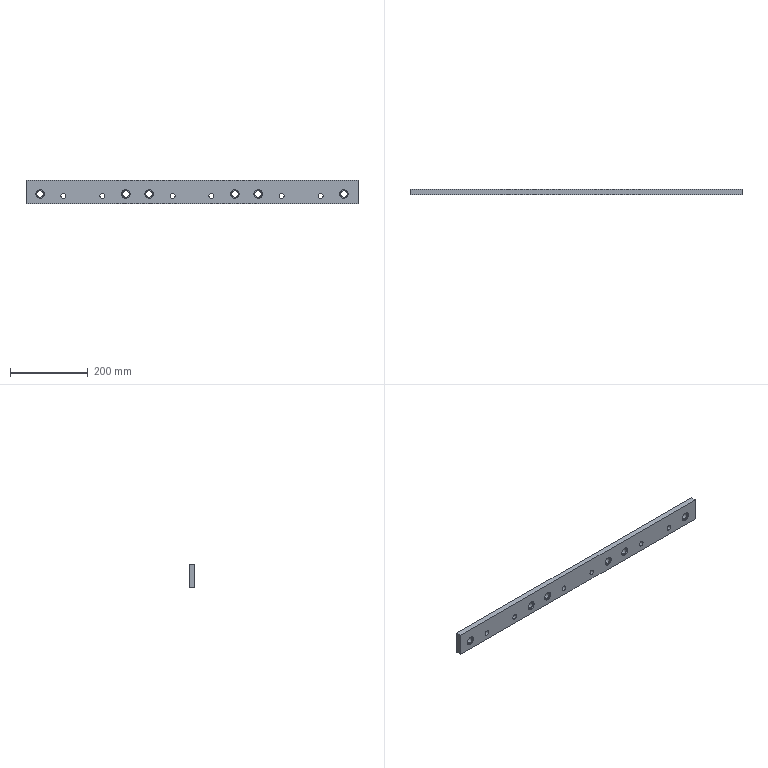Part | SolidWorks | features BaseBody 1 | 1 solid | 48 faces | box 852 x 14 x 60 mm | volume 682707 mm3 | cylinder 36 | plane 12 | commonest cylinder face diameters 13 x12 17 x12 22 x12
STEP:
#1=CARTESIAN_POINT('',(816.,3.,-43.5));
#2=VERTEX_POINT('',#1);
#3=CARTESIAN_POINT('',(816.,3.,-26.5));
#4=VERTEX_POINT('',#3);
#5=CARTESIAN_POINT('',(816.,3.,-35.));
#6=DIRECTION('',(0.,1.,0.));
#7=DIRECTION('',(0.,0.,1.));
#8=AXIS2_PLACEMENT_3D('',#5,#6,#7);
#9=CIRCLE('',#8,8.5);
#10=EDGE_CURVE('',#2,#4,#9,.T.);
#11=ORIENTED_EDGE('',*,*,#10,.F.);
#12=CARTESIAN_POINT('',(816.,14.,-43.5));
#13=VERTEX_POINT('',#12);
#14=CARTESIAN_POINT('',(816.,14.,-43.5));
#15=DIRECTION('',(0.,1.,0.));
#16=VECTOR('',#15,1000.);
#17=LINE('',#14,#16);
#18=EDGE_CURVE('',#2,#13,#17,.T.);
#19=ORIENTED_EDGE('',*,*,#18,.T.);
#20=CARTESIAN_POINT('',(816.,14.,-26.5));
#21=VERTEX_POINT('',#20);
#22=CARTESIAN_POINT('',(816.,14.,-35.));
#23=DIRECTION('',(0.,-1.,0.));
#24=DIRECTION('',(0.,0.,1.));
#25=AXIS2_PLACEMENT_3D('',#22,#23,#24);
#26=CIRCLE('',#25,8.5);
#27=EDGE_CURVE('',#21,#13,#26,.T.);
#28=ORIENTED_EDGE('',*,*,#27,.F.);
#29=CARTESIAN_POINT('',(816.,14.,-26.5));
#30=DIRECTION('',(0.,1.,0.));
#31=VECTOR('',#30,1000.);
#32=LINE('',#29,#31);
#33=EDGE_CURVE('',#4,#21,#32,.T.);
#34=ORIENTED_EDGE('',*,*,#33,.F.);
#35=EDGE_LOOP('',(#11,#19,#28,#34));
#36=FACE_OUTER_BOUND('',#35,.T.);
#37=CARTESIAN_POINT('',(816.,14.,-35.));
#38=DIRECTION('',(0.,1.,0.));
#39=DIRECTION('',(0.,0.,1.));
#40=AXIS2_PLACEMENT_3D('',#37,#38,#39);
#41=CYLINDRICAL_SURFACE('',#40,8.5);
#42=ADVANCED_FACE('',(#36),#41,.F.);
#43=CARTESIAN_POINT('',(536.,3.,-43.5));
#44=VERTEX_POINT('',#43);
#45=CARTESIAN_POINT('',(536.,3.,-26.5));
#46=VERTEX_POINT('',#45);
#47=CARTESIAN_POINT('',(536.,3.,-35.));
#48=DIRECTION('',(0.,1.,0.));
#49=DIRECTION('',(0.,0.,1.));
#50=AXIS2_PLACEMENT_3D('',#47,#48,#49);
#51=CIRCLE('',#50,8.5);
#52=EDGE_CURVE('',#44,#46,#51,.T.);
#53=ORIENTED_EDGE('',*,*,#52,.F.);
#54=CARTESIAN_POINT('',(536.,14.,-43.5));
#55=VERTEX_POINT('',#54);
#56=CARTESIAN_POINT('',(536.,14.,-43.5));
#57=DIRECTION('',(0.,1.,0.));
#58=VECTOR('',#57,1000.);
#59=LINE('',#56,#58);
#60=EDGE_CURVE('',#44,#55,#59,.T.);
#61=ORIENTED_EDGE('',*,*,#60,.T.);
#62=CARTESIAN_POINT('',(536.,14.,-26.5));
#63=VERTEX_POINT('',#62);
#64=CARTESIAN_POINT('',(536.,14.,-35.));
#65=DIRECTION('',(0.,-1.,0.));
#66=DIRECTION('',(0.,0.,1.));
#67=AXIS2_PLACEMENT_3D('',#64,#65,#66);
#68=CIRCLE('',#67,8.5);
#69=EDGE_CURVE('',#63,#55,#68,.T.);
#70=ORIENTED_EDGE('',*,*,#69,.F.);
#71=CARTESIAN_POINT('',(536.,14.,-26.5));
#72=DIRECTION('',(0.,1.,0.));
#73=VECTOR('',#72,1000.);
#74=LINE('',#71,#73);
#75=EDGE_CURVE('',#46,#63,#74,.T.);
#76=ORIENTED_EDGE('',*,*,#75,.F.);
#77=EDGE_LOOP('',(#53,#61,#70,#76));
#78=FACE_OUTER_BOUND('',#77,.T.);
#79=CARTESIAN_POINT('',(536.,14.,-35.));
#80=DIRECTION('',(0.,1.,0.));
#81=DIRECTION('',(0.,0.,1.));
#82=AXIS2_PLACEMENT_3D('',#79,#80,#81);
#83=CYLINDRICAL_SURFACE('',#82,8.5);
#84=ADVANCED_FACE('',(#78),#83,.F.);
#85=CARTESIAN_POINT('',(256.,3.,-43.5));
#86=VERTEX_POINT('',#85);
#87=CARTESIAN_POINT('',(256.,3.,-26.5));
#88=VERTEX_POINT('',#87);
#89=CARTESIAN_POINT('',(256.,3.,-35.));
#90=DIRECTION('',(0.,1.,0.));
#91=DIRECTION('',(0.,0.,1.));
#92=AXIS2_PLACEMENT_3D('',#89,#90,#91);
#93=CIRCLE('',#92,8.5);
#94=EDGE_CURVE('',#86,#88,#93,.T.);
#95=ORIENTED_EDGE('',*,*,#94,.F.);
#96=CARTESIAN_POINT('',(256.,14.,-43.5));
#97=VERTEX_POINT('',#96);
#98=CARTESIAN_POINT('',(256.,14.,-43.5));
#99=DIRECTION('',(0.,1.,0.));
#100=VECTOR('',#99,1000.);
#101=LINE('',#98,#100);
#102=EDGE_CURVE('',#86,#97,#101,.T.);
#103=ORIENTED_EDGE('',*,*,#102,.T.);
#104=CARTESIAN_POINT('',(256.,14.,-26.5));
#105=VERTEX_POINT('',#104);
#106=CARTESIAN_POINT('',(256.,14.,-35.));
#107=DIRECTION('',(0.,-1.,0.));
#108=DIRECTION('',(0.,0.,1.));
#109=AXIS2_PLACEMENT_3D('',#106,#107,#108);
#110=CIRCLE('',#109,8.5);
#111=EDGE_CURVE('',#105,#97,#110,.T.);
#112=ORIENTED_EDGE('',*,*,#111,.F.);
#113=CARTESIAN_POINT('',(256.,14.,-26.5));
#114=DIRECTION('',(0.,1.,0.));
#115=VECTOR('',#114,1000.);
#116=LINE('',#113,#115);
#117=EDGE_CURVE('',#88,#105,#116,.T.);
#118=ORIENTED_EDGE('',*,*,#117,.F.);
#119=EDGE_LOOP('',(#95,#103,#112,#118));
#120=FACE_OUTER_BOUND('',#119,.T.);
#121=CARTESIAN_POINT('',(256.,14.,-35.));
#122=DIRECTION('',(0.,1.,0.));
#123=DIRECTION('',(0.,0.,1.));
#124=AXIS2_PLACEMENT_3D('',#121,#122,#123);
#125=CYLINDRICAL_SURFACE('',#124,8.5);
#126=ADVANCED_FACE('',(#120),#125,.F.);
#127=CARTESIAN_POINT('',(756.,0.,-46.5));
#128=VERTEX_POINT('',#127);
#129=CARTESIAN_POINT('',(756.,0.,-33.5));
#130=VERTEX_POINT('',#129);
#131=CARTESIAN_POINT('',(756.,0.,-40.));
#132=DIRECTION('',(0.,1.,0.));
#133=DIRECTION('',(0.,0.,1.));
#134=AXIS2_PLACEMENT_3D('',#131,#132,#133);
#135=CIRCLE('',#134,6.5);
#136=EDGE_CURVE('',#128,#130,#135,.T.);
#137=ORIENTED_EDGE('',*,*,#136,.F.);
#138=CARTESIAN_POINT('',(756.,14.,-46.5));
#139=VERTEX_POINT('',#138);
#140=CARTESIAN_POINT('',(756.,14.,-46.5));
#141=DIRECTION('',(0.,1.,0.));
#142=VECTOR('',#141,1000.);
#143=LINE('',#140,#142);
#144=EDGE_CURVE('',#128,#139,#143,.T.);
#145=ORIENTED_EDGE('',*,*,#144,.T.);
#146=CARTESIAN_POINT('',(756.,14.,-33.5));
#147=VERTEX_POINT('',#146);
#148=CARTESIAN_POINT('',(756.,14.,-40.));
#149=DIRECTION('',(0.,-1.,0.));
#150=DIRECTION('',(0.,0.,1.));
#151=AXIS2_PLACEMENT_3D('',#148,#149,#150);
#152=CIRCLE('',#151,6.5);
#153=EDGE_CURVE('',#147,#139,#152,.T.);
#154=ORIENTED_EDGE('',*,*,#153,.F.);
#155=CARTESIAN_POINT('',(756.,14.,-33.5));
#156=DIRECTION('',(0.,1.,0.));
#157=VECTOR('',#156,1000.);
#158=LINE('',#155,#157);
#159=EDGE_CURVE('',#130,#147,#158,.T.);
#160=ORIENTED_EDGE('',*,*,#159,.F.);
#161=EDGE_LOOP('',(#137,#145,#154,#160));
#162=FACE_OUTER_BOUND('',#161,.T.);
#163=CARTESIAN_POINT('',(756.,14.,-40.));
#164=DIRECTION('',(0.,1.,0.));
#165=DIRECTION('',(0.,0.,1.));
#166=AXIS2_PLACEMENT_3D('',#163,#164,#165);
#167=CYLINDRICAL_SURFACE('',#166,6.5);
#168=ADVANCED_FACE('',(#162),#167,.F.);
#169=CARTESIAN_POINT('',(476.,0.,-46.5));
#170=VERTEX_POINT('',#169);
#171=CARTESIAN_POINT('',(476.,0.,-33.5));
#172=VERTEX_POINT('',#171);
#173=CARTESIAN_POINT('',(476.,0.,-40.));
#174=DIRECTION('',(0.,1.,0.));
#175=DIRECTION('',(0.,0.,1.));
#176=AXIS2_PLACEMENT_3D('',#173,#174,#175);
#177=CIRCLE('',#176,6.5);
#178=EDGE_CURVE('',#170,#172,#177,.T.);
#179=ORIENTED_EDGE('',*,*,#178,.F.);
#180=CARTESIAN_POINT('',(476.,14.,-46.5));
#181=VERTEX_POINT('',#180);
#182=CARTESIAN_POINT('',(476.,14.,-46.5));
#183=DIRECTION('',(0.,1.,0.));
#184=VECTOR('',#183,1000.);
#185=LINE('',#182,#184);
#186=EDGE_CURVE('',#170,#181,#185,.T.);
#187=ORIENTED_EDGE('',*,*,#186,.T.);
#188=CARTESIAN_POINT('',(476.,14.,-33.5));
#189=VERTEX_POINT('',#188);
#190=CARTESIAN_POINT('',(476.,14.,-40.));
#191=DIRECTION('',(0.,-1.,0.));
#192=DIRECTION('',(0.,0.,1.));
#193=AXIS2_PLACEMENT_3D('',#190,#191,#192);
#194=CIRCLE('',#193,6.5);
#195=EDGE_CURVE('',#189,#181,#194,.T.);
#196=ORIENTED_EDGE('',*,*,#195,.F.);
#197=CARTESIAN_POINT('',(476.,14.,-33.5));
#198=DIRECTION('',(0.,1.,0.));
#199=VECTOR('',#198,1000.);
#200=LINE('',#197,#199);
#201=EDGE_CURVE('',#172,#189,#200,.T.);
#202=ORIENTED_EDGE('',*,*,#201,.F.);
#203=EDGE_LOOP('',(#179,#187,#196,#202));
#204=FACE_OUTER_BOUND('',#203,.T.);
#205=CARTESIAN_POINT('',(476.,14.,-40.));
#206=DIRECTION('',(0.,1.,0.));
#207=DIRECTION('',(0.,0.,1.));
#208=AXIS2_PLACEMENT_3D('',#205,#206,#207);
#209=CYLINDRICAL_SURFACE('',#208,6.5);
#210=ADVANCED_FACE('',(#204),#209,.F.);
#211=CARTESIAN_POINT('',(196.,0.,-46.5));
#212=VERTEX_POINT('',#211);
#213=CARTESIAN_POINT('',(196.,0.,-33.5));
#214=VERTEX_POINT('',#213);
#215=CARTESIAN_POINT('',(196.,0.,-40.));
#216=DIRECTION('',(0.,1.,0.));
#217=DIRECTION('',(0.,0.,1.));
#218=AXIS2_PLACEMENT_3D('',#215,#216,#217);
#219=CIRCLE('',#218,6.5);
#220=EDGE_CURVE('',#212,#214,#219,.T.);
#221=ORIENTED_EDGE('',*,*,#220,.F.);
#222=CARTESIAN_POINT('',(196.,14.,-46.5));
#223=VERTEX_POINT('',#222);
#224=CARTESIAN_POINT('',(196.,14.,-46.5));
#225=DIRECTION('',(0.,1.,0.));
#226=VECTOR('',#225,1000.);
#227=LINE('',#224,#226);
#228=EDGE_CURVE('',#212,#223,#227,.T.);
#229=ORIENTED_EDGE('',*,*,#228,.T.);
#230=CARTESIAN_POINT('',(196.,14.,-33.5));
#231=VERTEX_POINT('',#230);
#232=CARTESIAN_POINT('',(196.,14.,-40.));
#233=DIRECTION('',(0.,-1.,0.));
#234=DIRECTION('',(0.,0.,1.));
#235=AXIS2_PLACEMENT_3D('',#232,#233,#234);
#236=CIRCLE('',#235,6.5);
#237=EDGE_CURVE('',#231,#223,#236,.T.);
#238=ORIENTED_EDGE('',*,*,#237,.F.);
#239=CARTESIAN_POINT('',(196.,14.,-33.5));
#240=DIRECTION('',(0.,1.,0.));
#241=VECTOR('',#240,1000.);
#242=LINE('',#239,#241);
#243=EDGE_CURVE('',#214,#231,#242,.T.);
#244=ORIENTED_EDGE('',*,*,#243,.F.);
#245=EDGE_LOOP('',(#221,#229,#238,#244));
#246=FACE_OUTER_BOUND('',#245,.T.);
#247=CARTESIAN_POINT('',(196.,14.,-40.));
#248=DIRECTION('',(0.,1.,0.));
#249=DIRECTION('',(0.,0.,1.));
#250=AXIS2_PLACEMENT_3D('',#247,#248,#249);
#251=CYLINDRICAL_SURFACE('',#250,6.5);
#252=ADVANCED_FACE('',(#246),#251,.F.);
#253=CARTESIAN_POINT('',(96.,0.,-46.5));
#254=VERTEX_POINT('',#253);
#255=CARTESIAN_POINT('',(96.,0.,-33.5));
#256=VERTEX_POINT('',#255);
#257=CARTESIAN_POINT('',(96.,0.,-40.));
#258=DIRECTION('',(0.,1.,0.));
#259=DIRECTION('',(0.,0.,1.));
#260=AXIS2_PLACEMENT_3D('',#257,#258,#259);
#261=CIRCLE('',#260,6.5);
#262=EDGE_CURVE('',#254,#256,#261,.T.);
#263=ORIENTED_EDGE('',*,*,#262,.F.);
#264=CARTESIAN_POINT('',(96.,14.,-46.5));
#265=VERTEX_POINT('',#264);
#266=CARTESIAN_POINT('',(96.,14.,-46.5));
#267=DIRECTION('',(0.,1.,0.));
#268=VECTOR('',#267,1000.);
#269=LINE('',#266,#268);
#270=EDGE_CURVE('',#254,#265,#269,.T.);
#271=ORIENTED_EDGE('',*,*,#270,.T.);
#272=CARTESIAN_POINT('',(96.,14.,-33.5));
#273=VERTEX_POINT('',#272);
#274=CARTESIAN_POINT('',(96.,14.,-40.));
#275=DIRECTION('',(0.,-1.,0.));
#276=DIRECTION('',(0.,0.,1.));
#277=AXIS2_PLACEMENT_3D('',#274,#275,#276);
#278=CIRCLE('',#277,6.5);
#279=EDGE_CURVE('',#273,#265,#278,.T.);
#280=ORIENTED_EDGE('',*,*,#279,.F.);
#281=CARTESIAN_POINT('',(96.,14.,-33.5));
#282=DIRECTION('',(0.,1.,0.));
#283=VECTOR('',#282,1000.);
#284=LINE('',#281,#283);
#285=EDGE_CURVE('',#256,#273,#284,.T.);
#286=ORIENTED_EDGE('',*,*,#285,.F.);
#287=EDGE_LOOP('',(#263,#271,#280,#286));
#288=FACE_OUTER_BOUND('',#287,.T.);
#289=CARTESIAN_POINT('',(96.,14.,-40.));
#290=DIRECTION('',(0.,1.,0.));
#291=DIRECTION('',(0.,0.,1.));
#292=AXIS2_PLACEMENT_3D('',#289,#290,#291);
#293=CYLINDRICAL_SURFACE('',#292,6.5);
#294=ADVANCED_FACE('',(#288),#293,.F.);
#295=CARTESIAN_POINT('',(376.,0.,-46.5));
#296=VERTEX_POINT('',#295);
#297=CARTESIAN_POINT('',(376.,0.,-33.5));
#298=VERTEX_POINT('',#297);
#299=CARTESIAN_POINT('',(376.,0.,-40.));
#300=DIRECTION('',(0.,1.,0.));
#301=DIRECTION('',(0.,0.,1.));
#302=AXIS2_PLACEMENT_3D('',#299,#300,#301);
#303=CIRCLE('',#302,6.5);
#304=EDGE_CURVE('',#296,#298,#303,.T.);
#305=ORIENTED_EDGE('',*,*,#304,.F.);
#306=CARTESIAN_POINT('',(376.,14.,-46.5));
#307=VERTEX_POINT('',#306);
#308=CARTESIAN_POINT('',(376.,14.,-46.5));
#309=DIRECTION('',(0.,1.,0.));
#310=VECTOR('',#309,1000.);
#311=LINE('',#308,#310);
#312=EDGE_CURVE('',#296,#307,#311,.T.);
#313=ORIENTED_EDGE('',*,*,#312,.T.);
#314=CARTESIAN_POINT('',(376.,14.,-33.5));
#315=VERTEX_POINT('',#314);
#316=CARTESIAN_POINT('',(376.,14.,-40.));
#317=DIRECTION('',(0.,-1.,0.));
#318=DIRECTION('',(0.,0.,1.));
#319=AXIS2_PLACEMENT_3D('',#316,#317,#318);
#320=CIRCLE('',#319,6.5);
#321=EDGE_CURVE('',#315,#307,#320,.T.);
#322=ORIENTED_EDGE('',*,*,#321,.F.);
#323=CARTESIAN_POINT('',(376.,14.,-33.5));
#324=DIRECTION('',(0.,1.,0.));
#325=VECTOR('',#324,1000.);
#326=LINE('',#323,#325);
#327=EDGE_CURVE('',#298,#315,#326,.T.);
#328=ORIENTED_EDGE('',*,*,#327,.F.);
#329=EDGE_LOOP('',(#305,#313,#322,#328));
#330=FACE_OUTER_BOUND('',#329,.T.);
#331=CARTESIAN_POINT('',(376.,14.,-40.));
#332=DIRECTION('',(0.,1.,0.));
#333=DIRECTION('',(0.,0.,1.));
#334=AXIS2_PLACEMENT_3D('',#331,#332,#333);
#335=CYLINDRICAL_SURFACE('',#334,6.5);
#336=ADVANCED_FACE('',(#330),#335,.F.);
#337=CARTESIAN_POINT('',(656.,0.,-46.5));
#338=VERTEX_POINT('',#337);
#339=CARTESIAN_POINT('',(656.,0.,-33.5));
#340=VERTEX_POINT('',#339);
#341=CARTESIAN_POINT('',(656.,0.,-40.));
#342=DIRECTION('',(0.,1.,0.));
#343=DIRECTION('',(0.,0.,1.));
#344=AXIS2_PLACEMENT_3D('',#341,#342,#343);
#345=CIRCLE('',#344,6.5);
#346=EDGE_CURVE('',#338,#340,#345,.T.);
#347=ORIENTED_EDGE('',*,*,#346,.F.);
#348=CARTESIAN_POINT('',(656.,14.,-46.5));
#349=VERTEX_POINT('',#348);
#350=CARTESIAN_POINT('',(656.,14.,-46.5));
#351=DIRECTION('',(0.,1.,0.));
#352=VECTOR('',#351,1000.);
#353=LINE('',#350,#352);
#354=EDGE_CURVE('',#338,#349,#353,.T.);
#355=ORIENTED_EDGE('',*,*,#354,.T.);
#356=CARTESIAN_POINT('',(656.,14.,-33.5));
#357=VERTEX_POINT('',#356);
#358=CARTESIAN_POINT('',(656.,14.,-40.));
#359=DIRECTION('',(0.,-1.,0.));
#360=DIRECTION('',(0.,0.,1.));
#361=AXIS2_PLACEMENT_3D('',#358,#359,#360);
#362=CIRCLE('',#361,6.5);
#363=EDGE_CURVE('',#357,#349,#362,.T.);
#364=ORIENTED_EDGE('',*,*,#363,.F.);
#365=CARTESIAN_POINT('',(656.,14.,-33.5));
#366=DIRECTION('',(0.,1.,0.));
#367=VECTOR('',#366,1000.);
#368=LINE('',#365,#367);
#369=EDGE_CURVE('',#340,#357,#368,.T.);
#370=ORIENTED_EDGE('',*,*,#369,.F.);
#371=EDGE_LOOP('',(#347,#355,#364,#370));
#372=FACE_OUTER_BOUND('',#371,.T.);
#373=CARTESIAN_POINT('',(656.,14.,-40.));
#374=DIRECTION('',(0.,1.,0.));
#375=DIRECTION('',(0.,0.,1.));
#376=AXIS2_PLACEMENT_3D('',#373,#374,#375);
#377=CYLINDRICAL_SURFACE('',#376,6.5);
#378=ADVANCED_FACE('',(#372),#377,.F.);
#379=CARTESIAN_POINT('',(36.,3.,-43.5));
#380=VERTEX_POINT('',#379);
#381=CARTESIAN_POINT('',(36.,3.,-26.5));
#382=VERTEX_POINT('',#381);
#383=CARTESIAN_POINT('',(36.,3.,-35.));
#384=DIRECTION('',(0.,1.,0.));
#385=DIRECTION('',(0.,0.,1.));
#386=AXIS2_PLACEMENT_3D('',#383,#384,#385);
#387=CIRCLE('',#386,8.5);
#388=EDGE_CURVE('',#380,#382,#387,.T.);
#389=ORIENTED_EDGE('',*,*,#388,.F.);
#390=CARTESIAN_POINT('',(36.,14.,-43.5));
#391=VERTEX_POINT('',#390);
#392=CARTESIAN_POINT('',(36.,14.,-43.5));
#393=DIRECTION('',(0.,1.,0.));
#394=VECTOR('',#393,1000.);
#395=LINE('',#392,#394);
#396=EDGE_CURVE('',#380,#391,#395,.T.);
#397=ORIENTED_EDGE('',*,*,#396,.T.);
#398=CARTESIAN_POINT('',(36.,14.,-26.5));
#399=VERTEX_POINT('',#398);
#400=CARTESIAN_POINT('',(36.,14.,-35.));
#401=DIRECTION('',(0.,-1.,0.));
#402=DIRECTION('',(0.,0.,1.));
#403=AXIS2_PLACEMENT_3D('',#400,#401,#402);
#404=CIRCLE('',#403,8.5);
#405=EDGE_CURVE('',#399,#391,#404,.T.);
#406=ORIENTED_EDGE('',*,*,#405,.F.);
#407=CARTESIAN_POINT('',(36.,14.,-26.5));
#408=DIRECTION('',(0.,1.,0.));
#409=VECTOR('',#408,1000.);
#410=LINE('',#407,#409);
#411=EDGE_CURVE('',#382,#399,#410,.T.);
#412=ORIENTED_EDGE('',*,*,#411,.F.);
#413=EDGE_LOOP('',(#389,#397,#406,#412));
#414=FACE_OUTER_BOUND('',#413,.T.);
#415=CARTESIAN_POINT('',(36.,14.,-35.));
#416=DIRECTION('',(0.,1.,0.));
#417=DIRECTION('',(0.,0.,1.));
#418=AXIS2_PLACEMENT_3D('',#415,#416,#417);
#419=CYLINDRICAL_SURFACE('',#418,8.5);
#420=ADVANCED_FACE('',(#414),#419,.F.);
#421=CARTESIAN_POINT('',(316.,3.,-43.5));
#422=VERTEX_POINT('',#421);
#423=CARTESIAN_POINT('',(316.,3.,-26.5));
#424=VERTEX_POINT('',#423);
#425=CARTESIAN_POINT('',(316.,3.,-35.));
#426=DIRECTION('',(0.,1.,0.));
#427=DIRECTION('',(0.,0.,1.));
#428=AXIS2_PLACEMENT_3D('',#425,#426,#427);
#429=CIRCLE('',#428,8.5);
#430=EDGE_CURVE('',#422,#424,#429,.T.);
#431=ORIENTED_EDGE('',*,*,#430,.F.);
#432=CARTESIAN_POINT('',(316.,14.,-43.5));
#433=VERTEX_POINT('',#432);
#434=CARTESIAN_POINT('',(316.,14.,-43.5));
#435=DIRECTION('',(0.,1.,0.));
#436=VECTOR('',#435,1000.);
#437=LINE('',#434,#436);
#438=EDGE_CURVE('',#422,#433,#437,.T.);
#439=ORIENTED_EDGE('',*,*,#438,.T.);
#440=CARTESIAN_POINT('',(316.,14.,-26.5));
#441=VERTEX_POINT('',#440);
#442=CARTESIAN_POINT('',(316.,14.,-35.));
#443=DIRECTION('',(0.,-1.,0.));
#444=DIRECTION('',(0.,0.,1.));
#445=AXIS2_PLACEMENT_3D('',#442,#443,#444);
#446=CIRCLE('',#445,8.5);
#447=EDGE_CURVE('',#441,#433,#446,.T.);
#448=ORIENTED_EDGE('',*,*,#447,.F.);
#449=CARTESIAN_POINT('',(316.,14.,-26.5));
#450=DIRECTION('',(0.,1.,0.));
#451=VECTOR('',#450,1000.);
#452=LINE('',#449,#451);
#453=EDGE_CURVE('',#424,#441,#452,.T.);
#454=ORIENTED_EDGE('',*,*,#453,.F.);
#455=EDGE_LOOP('',(#431,#439,#448,#454));
#456=FACE_OUTER_BOUND('',#455,.T.);
#457=CARTESIAN_POINT('',(316.,14.,-35.));
#458=DIRECTION('',(0.,1.,0.));
#459=DIRECTION('',(0.,0.,1.));
#460=AXIS2_PLACEMENT_3D('',#457,#458,#459);
#461=CYLINDRICAL_SURFACE('',#460,8.5);
#462=ADVANCED_FACE('',(#456),#461,.F.);
#463=CARTESIAN_POINT('',(596.,3.,-43.5));
#464=VERTEX_POINT('',#463);
#465=CARTESIAN_POINT('',(596.,3.,-26.5));
#466=VERTEX_POINT('',#465);
#467=CARTESIAN_POINT('',(596.,3.,-35.));
#468=DIRECTION('',(0.,1.,0.));
#469=DIRECTION('',(0.,0.,1.));
#470=AXIS2_PLACEMENT_3D('',#467,#468,#469);
#471=CIRCLE('',#470,8.5);
#472=EDGE_CURVE('',#464,#466,#471,.T.);
#473=ORIENTED_EDGE('',*,*,#472,.F.);
#474=CARTESIAN_POINT('',(596.,14.,-43.5));
#475=VERTEX_POINT('',#474);
#476=CARTESIAN_POINT('',(596.,14.,-43.5));
#477=DIRECTION('',(0.,1.,0.));
#478=VECTOR('',#477,1000.);
#479=LINE('',#476,#478);
#480=EDGE_CURVE('',#464,#475,#479,.T.);
#481=ORIENTED_EDGE('',*,*,#480,.T.);
#482=CARTESIAN_POINT('',(596.,14.,-26.5));
#483=VERTEX_POINT('',#482);
#484=CARTESIAN_POINT('',(596.,14.,-35.));
#485=DIRECTION('',(0.,-1.,0.));
#486=DIRECTION('',(0.,0.,1.));
#487=AXIS2_PLACEMENT_3D('',#484,#485,#486);
#488=CIRCLE('',#487,8.5);
#489=EDGE_CURVE('',#483,#475,#488,.T.);
#490=ORIENTED_EDGE('',*,*,#489,.F.);
#491=CARTESIAN_POINT('',(596.,14.,-26.5));
#492=DIRECTION('',(0.,1.,0.));
#493=VECTOR('',#492,1000.);
#494=LINE('',#491,#493);
#495=EDGE_CURVE('',#466,#483,#494,.T.);
#496=ORIENTED_EDGE('',*,*,#495,.F.);
#497=EDGE_LOOP('',(#473,#481,#490,#496));
#498=FACE_OUTER_BOUND('',#497,.T.);
#499=CARTESIAN_POINT('',(596.,14.,-35.));
#500=DIRECTION('',(0.,1.,0.));
#501=DIRECTION('',(0.,0.,1.));
#502=AXIS2_PLACEMENT_3D('',#499,#500,#501);
#503=CYLINDRICAL_SURFACE('',#502,8.5);
#504=ADVANCED_FACE('',(#498),#503,.F.);
#505=CARTESIAN_POINT('',(816.,0.,-46.));
#506=VERTEX_POINT('',#505);
#507=CARTESIAN_POINT('',(816.,0.,-24.));
#508=VERTEX_POINT('',#507);
#509=CARTESIAN_POINT('',(816.,0.,-35.));
#510=DIRECTION('',(0.,1.,0.));
#511=DIRECTION('',(0.,0.,1.));
#512=AXIS2_PLACEMENT_3D('',#509,#510,#511);
#513=CIRCLE('',#512,11.);
#514=EDGE_CURVE('',#506,#508,#513,.T.);
#515=ORIENTED_EDGE('',*,*,#514,.F.);
#516=CARTESIAN_POINT('',(816.,3.,-46.));
#517=VERTEX_POINT('',#516);
#518=CARTESIAN_POINT('',(816.,0.,-46.));
#519=DIRECTION('',(0.,1.,0.));
#520=VECTOR('',#519,1000.);
#521=LINE('',#518,#520);
#522=EDGE_CURVE('',#506,#517,#521,.T.);
#523=ORIENTED_EDGE('',*,*,#522,.T.);
#524=CARTESIAN_POINT('',(816.,3.,-24.));
#525=VERTEX_POINT('',#524);
#526=CARTESIAN_POINT('',(816.,3.,-35.));
#527=DIRECTION('',(0.,-1.,0.));
#528=DIRECTION('',(0.,0.,1.));
#529=AXIS2_PLACEMENT_3D('',#526,#527,#528);
#530=CIRCLE('',#529,11.);
#531=EDGE_CURVE('',#525,#517,#530,.T.);
#532=ORIENTED_EDGE('',*,*,#531,.F.);
#533=CARTESIAN_POINT('',(816.,0.,-24.));
#534=DIRECTION('',(0.,1.,0.));
#535=VECTOR('',#534,1000.);
#536=LINE('',#533,#535);
#537=EDGE_CURVE('',#508,#525,#536,.T.);
#538=ORIENTED_EDGE('',*,*,#537,.F.);
#539=EDGE_LOOP('',(#515,#523,#532,#538));
#540=FACE_OUTER_BOUND('',#539,.T.);
#541=CARTESIAN_POINT('',(816.,0.,-35.));
#542=DIRECTION('',(0.,1.,0.));
#543=DIRECTION('',(0.,0.,1.));
#544=AXIS2_PLACEMENT_3D('',#541,#542,#543);
#545=CYLINDRICAL_SURFACE('',#544,11.);
#546=ADVANCED_FACE('',(#540),#545,.F.);
#547=CARTESIAN_POINT('',(536.,0.,-46.));
#548=VERTEX_POINT('',#547);
#549=CARTESIAN_POINT('',(536.,0.,-24.));
#550=VERTEX_POINT('',#549);
#551=CARTESIAN_POINT('',(536.,0.,-35.));
#552=DIRECTION('',(0.,1.,0.));
#553=DIRECTION('',(0.,0.,1.));
#554=AXIS2_PLACEMENT_3D('',#551,#552,#553);
#555=CIRCLE('',#554,11.);
#556=EDGE_CURVE('',#548,#550,#555,.T.);
#557=ORIENTED_EDGE('',*,*,#556,.F.);
#558=CARTESIAN_POINT('',(536.,3.,-46.));
#559=VERTEX_POINT('',#558);
#560=CARTESIAN_POINT('',(536.,0.,-46.));
#561=DIRECTION('',(0.,1.,0.));
#562=VECTOR('',#561,1000.);
#563=LINE('',#560,#562);
#564=EDGE_CURVE('',#548,#559,#563,.T.);
#565=ORIENTED_EDGE('',*,*,#564,.T.);
#566=CARTESIAN_POINT('',(536.,3.,-24.));
#567=VERTEX_POINT('',#566);
#568=CARTESIAN_POINT('',(536.,3.,-35.));
#569=DIRECTION('',(0.,-1.,0.));
#570=DIRECTION('',(0.,0.,1.));
#571=AXIS2_PLACEMENT_3D('',#568,#569,#570);
#572=CIRCLE('',#571,11.);
#573=EDGE_CURVE('',#567,#559,#572,.T.);
#574=ORIENTED_EDGE('',*,*,#573,.F.);
#575=CARTESIAN_POINT('',(536.,0.,-24.));
#576=DIRECTION('',(0.,1.,0.));
#577=VECTOR('',#576,1000.);
#578=LINE('',#575,#577);
#579=EDGE_CURVE('',#550,#567,#578,.T.);
#580=ORIENTED_EDGE('',*,*,#579,.F.);
#581=EDGE_LOOP('',(#557,#565,#574,#580));
#582=FACE_OUTER_BOUND('',#581,.T.);
#583=CARTESIAN_POINT('',(536.,0.,-35.));
#584=DIRECTION('',(0.,1.,0.));
#585=DIRECTION('',(0.,0.,1.));
#586=AXIS2_PLACEMENT_3D('',#583,#584,#585);
#587=CYLINDRICAL_SURFACE('',#586,11.);
#588=ADVANCED_FACE('',(#582),#587,.F.);
#589=CARTESIAN_POINT('',(256.,0.,-46.));
#590=VERTEX_POINT('',#589);
#591=CARTESIAN_POINT('',(256.,0.,-24.));
#592=VERTEX_POINT('',#591);
#593=CARTESIAN_POINT('',(256.,0.,-35.));
#594=DIRECTION('',(0.,1.,0.));
#595=DIRECTION('',(0.,0.,1.));
#596=AXIS2_PLACEMENT_3D('',#593,#594,#595);
#597=CIRCLE('',#596,11.);
#598=EDGE_CURVE('',#590,#592,#597,.T.);
#599=ORIENTED_EDGE('',*,*,#598,.F.);
#600=CARTESIAN_POINT('',(256.,3.,-46.));
#601=VERTEX_POINT('',#600);
#602=CARTESIAN_POINT('',(256.,0.,-46.));
#603=DIRECTION('',(0.,1.,0.));
#604=VECTOR('',#603,1000.);
#605=LINE('',#602,#604);
#606=EDGE_CURVE('',#590,#601,#605,.T.);
#607=ORIENTED_EDGE('',*,*,#606,.T.);
#608=CARTESIAN_POINT('',(256.,3.,-24.));
#609=VERTEX_POINT('',#608);
#610=CARTESIAN_POINT('',(256.,3.,-35.));
#611=DIRECTION('',(0.,-1.,0.));
#612=DIRECTION('',(0.,0.,1.));
#613=AXIS2_PLACEMENT_3D('',#610,#611,#612);
#614=CIRCLE('',#613,11.);
#615=EDGE_CURVE('',#609,#601,#614,.T.);
#616=ORIENTED_EDGE('',*,*,#615,.F.);
#617=CARTESIAN_POINT('',(256.,0.,-24.));
#618=DIRECTION('',(0.,1.,0.));
#619=VECTOR('',#618,1000.);
#620=LINE('',#617,#619);
#621=EDGE_CURVE('',#592,#609,#620,.T.);
#622=ORIENTED_EDGE('',*,*,#621,.F.);
#623=EDGE_LOOP('',(#599,#607,#616,#622));
#624=FACE_OUTER_BOUND('',#623,.T.);
#625=CARTESIAN_POINT('',(256.,0.,-35.));
#626=DIRECTION('',(0.,1.,0.));
#627=DIRECTION('',(0.,0.,1.));
#628=AXIS2_PLACEMENT_3D('',#625,#626,#627);
#629=CYLINDRICAL_SURFACE('',#628,11.);
#630=ADVANCED_FACE('',(#624),#629,.F.);
#631=CARTESIAN_POINT('',(596.,0.,-46.));
#632=VERTEX_POINT('',#631);
#633=CARTESIAN_POINT('',(596.,0.,-24.));
#634=VERTEX_POINT('',#633);
#635=CARTESIAN_POINT('',(596.,0.,-35.));
#636=DIRECTION('',(0.,1.,0.));
#637=DIRECTION('',(0.,0.,1.));
#638=AXIS2_PLACEMENT_3D('',#635,#636,#637);
#639=CIRCLE('',#638,11.);
#640=EDGE_CURVE('',#632,#634,#639,.T.);
#641=ORIENTED_EDGE('',*,*,#640,.F.);
#642=CARTESIAN_POINT('',(596.,3.,-46.));
#643=VERTEX_POINT('',#642);
#644=CARTESIAN_POINT('',(596.,0.,-46.));
#645=DIRECTION('',(0.,1.,0.));
#646=VECTOR('',#645,1000.);
#647=LINE('',#644,#646);
#648=EDGE_CURVE('',#632,#643,#647,.T.);
#649=ORIENTED_EDGE('',*,*,#648,.T.);
#650=CARTESIAN_POINT('',(596.,3.,-24.));
#651=VERTEX_POINT('',#650);
#652=CARTESIAN_POINT('',(596.,3.,-35.));
#653=DIRECTION('',(0.,-1.,0.));
#654=DIRECTION('',(0.,0.,1.));
#655=AXIS2_PLACEMENT_3D('',#652,#653,#654);
#656=CIRCLE('',#655,11.);
#657=EDGE_CURVE('',#651,#643,#656,.T.);
#658=ORIENTED_EDGE('',*,*,#657,.F.);
#659=CARTESIAN_POINT('',(596.,0.,-24.));
#660=DIRECTION('',(0.,1.,0.));
#661=VECTOR('',#660,1000.);
#662=LINE('',#659,#661);
#663=EDGE_CURVE('',#634,#651,#662,.T.);
#664=ORIENTED_EDGE('',*,*,#663,.F.);
#665=EDGE_LOOP('',(#641,#649,#658,#664));
#666=FACE_OUTER_BOUND('',#665,.T.);
#667=CARTESIAN_POINT('',(596.,0.,-35.));
#668=DIRECTION('',(0.,1.,0.));
#669=DIRECTION('',(0.,0.,1.));
#670=AXIS2_PLACEMENT_3D('',#667,#668,#669);
#671=CYLINDRICAL_SURFACE('',#670,11.);
#672=ADVANCED_FACE('',(#666),#671,.F.);
#673=CARTESIAN_POINT('',(316.,0.,-46.));
#674=VERTEX_POINT('',#673);
#675=CARTESIAN_POINT('',(316.,0.,-24.));
#676=VERTEX_POINT('',#675);
#677=CARTESIAN_POINT('',(316.,0.,-35.));
#678=DIRECTION('',(0.,1.,0.));
#679=DIRECTION('',(0.,0.,1.));
#680=AXIS2_PLACEMENT_3D('',#677,#678,#679);
#681=CIRCLE('',#680,11.);
#682=EDGE_CURVE('',#674,#676,#681,.T.);
#683=ORIENTED_EDGE('',*,*,#682,.F.);
#684=CARTESIAN_POINT('',(316.,3.,-46.));
#685=VERTEX_POINT('',#684);
#686=CARTESIAN_POINT('',(316.,0.,-46.));
#687=DIRECTION('',(0.,1.,0.));
#688=VECTOR('',#687,1000.);
#689=LINE('',#686,#688);
#690=EDGE_CURVE('',#674,#685,#689,.T.);
#691=ORIENTED_EDGE('',*,*,#690,.T.);
#692=CARTESIAN_POINT('',(316.,3.,-24.));
#693=VERTEX_POINT('',#692);
#694=CARTESIAN_POINT('',(316.,3.,-35.));
#695=DIRECTION('',(0.,-1.,0.));
#696=DIRECTION('',(0.,0.,1.));
#697=AXIS2_PLACEMENT_3D('',#694,#695,#696);
#698=CIRCLE('',#697,11.);
#699=EDGE_CURVE('',#693,#685,#698,.T.);
#700=ORIENTED_EDGE('',*,*,#699,.F.);
#701=CARTESIAN_POINT('',(316.,0.,-24.));
#702=DIRECTION('',(0.,1.,0.));
#703=VECTOR('',#702,1000.);
#704=LINE('',#701,#703);
#705=EDGE_CURVE('',#676,#693,#704,.T.);
#706=ORIENTED_EDGE('',*,*,#705,.F.);
#707=EDGE_LOOP('',(#683,#691,#700,#706));
#708=FACE_OUTER_BOUND('',#707,.T.);
#709=CARTESIAN_POINT('',(316.,0.,-35.));
#710=DIRECTION('',(0.,1.,0.));
#711=DIRECTION('',(0.,0.,1.));
#712=AXIS2_PLACEMENT_3D('',#709,#710,#711);
#713=CYLINDRICAL_SURFACE('',#712,11.);
#714=ADVANCED_FACE('',(#708),#713,.F.);
#715=CARTESIAN_POINT('',(36.,0.,-46.));
#716=VERTEX_POINT('',#715);
#717=CARTESIAN_POINT('',(36.,0.,-24.));
#718=VERTEX_POINT('',#717);
#719=CARTESIAN_POINT('',(36.,0.,-35.));
#720=DIRECTION('',(0.,1.,0.));
#721=DIRECTION('',(0.,0.,1.));
#722=AXIS2_PLACEMENT_3D('',#719,#720,#721);
#723=CIRCLE('',#722,11.);
#724=EDGE_CURVE('',#716,#718,#723,.T.);
#725=ORIENTED_EDGE('',*,*,#724,.F.);
#726=CARTESIAN_POINT('',(36.,3.,-46.));
#727=VERTEX_POINT('',#726);
#728=CARTESIAN_POINT('',(36.,0.,-46.));
#729=DIRECTION('',(0.,1.,0.));
#730=VECTOR('',#729,1000.);
#731=LINE('',#728,#730);
#732=EDGE_CURVE('',#716,#727,#731,.T.);
#733=ORIENTED_EDGE('',*,*,#732,.T.);
#734=CARTESIAN_POINT('',(36.,3.,-24.));
#735=VERTEX_POINT('',#734);
#736=CARTESIAN_POINT('',(36.,3.,-35.));
#737=DIRECTION('',(0.,-1.,0.));
#738=DIRECTION('',(0.,0.,1.));
#739=AXIS2_PLACEMENT_3D('',#736,#737,#738);
#740=CIRCLE('',#739,11.);
#741=EDGE_CURVE('',#735,#727,#740,.T.);
#742=ORIENTED_EDGE('',*,*,#741,.F.);
#743=CARTESIAN_POINT('',(36.,0.,-24.));
#744=DIRECTION('',(0.,1.,0.));
#745=VECTOR('',#744,1000.);
#746=LINE('',#743,#745);
#747=EDGE_CURVE('',#718,#735,#746,.T.);
#748=ORIENTED_EDGE('',*,*,#747,.F.);
#749=EDGE_LOOP('',(#725,#733,#742,#748));
#750=FACE_OUTER_BOUND('',#749,.T.);
#751=CARTESIAN_POINT('',(36.,0.,-35.));
#752=DIRECTION('',(0.,1.,0.));
#753=DIRECTION('',(0.,0.,1.));
#754=AXIS2_PLACEMENT_3D('',#751,#752,#753);
#755=CYLINDRICAL_SURFACE('',#754,11.);
#756=ADVANCED_FACE('',(#750),#755,.F.);
#757=ORIENTED_EDGE('',*,*,#27,.T.);
#758=CARTESIAN_POINT('',(816.,14.,-35.));
#759=DIRECTION('',(0.,-1.,0.));
#760=DIRECTION('',(0.,0.,1.));
#761=AXIS2_PLACEMENT_3D('',#758,#759,#760);
#762=CIRCLE('',#761,8.5);
#763=EDGE_CURVE('',#13,#21,#762,.T.);
#764=ORIENTED_EDGE('',*,*,#763,.T.);
#765=EDGE_LOOP('',(#757,#764));
#766=FACE_BOUND('',#765,.T.);
#767=ORIENTED_EDGE('',*,*,#69,.T.);
#768=CARTESIAN_POINT('',(536.,14.,-35.));
#769=DIRECTION('',(0.,-1.,0.));
#770=DIRECTION('',(0.,0.,1.));
#771=AXIS2_PLACEMENT_3D('',#768,#769,#770);
#772=CIRCLE('',#771,8.5);
#773=EDGE_CURVE('',#55,#63,#772,.T.);
#774=ORIENTED_EDGE('',*,*,#773,.T.);
#775=EDGE_LOOP('',(#767,#774));
#776=FACE_BOUND('',#775,.T.);
#777=ORIENTED_EDGE('',*,*,#111,.T.);
#778=CARTESIAN_POINT('',(256.,14.,-35.));
#779=DIRECTION('',(0.,-1.,0.));
#780=DIRECTION('',(0.,0.,1.));
#781=AXIS2_PLACEMENT_3D('',#778,#779,#780);
#782=CIRCLE('',#781,8.5);
#783=EDGE_CURVE('',#97,#105,#782,.T.);
#784=ORIENTED_EDGE('',*,*,#783,.T.);
#785=EDGE_LOOP('',(#777,#784));
#786=FACE_BOUND('',#785,.T.);
#787=ORIENTED_EDGE('',*,*,#153,.T.);
#788=CARTESIAN_POINT('',(756.,14.,-40.));
#789=DIRECTION('',(0.,-1.,0.));
#790=DIRECTION('',(0.,0.,1.));
#791=AXIS2_PLACEMENT_3D('',#788,#789,#790);
#792=CIRCLE('',#791,6.5);
#793=EDGE_CURVE('',#139,#147,#792,.T.);
#794=ORIENTED_EDGE('',*,*,#793,.T.);
#795=EDGE_LOOP('',(#787,#794));
#796=FACE_BOUND('',#795,.T.);
#797=ORIENTED_EDGE('',*,*,#195,.T.);
#798=CARTESIAN_POINT('',(476.,14.,-40.));
#799=DIRECTION('',(0.,-1.,0.));
#800=DIRECTION('',(0.,0.,1.));
#801=AXIS2_PLACEMENT_3D('',#798,#799,#800);
#802=CIRCLE('',#801,6.5);
#803=EDGE_CURVE('',#181,#189,#802,.T.);
#804=ORIENTED_EDGE('',*,*,#803,.T.);
#805=EDGE_LOOP('',(#797,#804));
#806=FACE_BOUND('',#805,.T.);
#807=ORIENTED_EDGE('',*,*,#237,.T.);
#808=CARTESIAN_POINT('',(196.,14.,-40.));
#809=DIRECTION('',(0.,-1.,0.));
#810=DIRECTION('',(0.,0.,1.));
#811=AXIS2_PLACEMENT_3D('',#808,#809,#810);
#812=CIRCLE('',#811,6.5);
#813=EDGE_CURVE('',#223,#231,#812,.T.);
#814=ORIENTED_EDGE('',*,*,#813,.T.);
#815=EDGE_LOOP('',(#807,#814));
#816=FACE_BOUND('',#815,.T.);
#817=ORIENTED_EDGE('',*,*,#279,.T.);
#818=CARTESIAN_POINT('',(96.,14.,-40.));
#819=DIRECTION('',(0.,-1.,0.));
#820=DIRECTION('',(0.,0.,1.));
#821=AXIS2_PLACEMENT_3D('',#818,#819,#820);
#822=CIRCLE('',#821,6.5);
#823=EDGE_CURVE('',#265,#273,#822,.T.);
#824=ORIENTED_EDGE('',*,*,#823,.T.);
#825=EDGE_LOOP('',(#817,#824));
#826=FACE_BOUND('',#825,.T.);
#827=ORIENTED_EDGE('',*,*,#321,.T.);
#828=CARTESIAN_POINT('',(376.,14.,-40.));
#829=DIRECTION('',(0.,-1.,0.));
#830=DIRECTION('',(0.,0.,1.));
#831=AXIS2_PLACEMENT_3D('',#828,#829,#830);
#832=CIRCLE('',#831,6.5);
#833=EDGE_CURVE('',#307,#315,#832,.T.);
#834=ORIENTED_EDGE('',*,*,#833,.T.);
#835=EDGE_LOOP('',(#827,#834));
#836=FACE_BOUND('',#835,.T.);
#837=ORIENTED_EDGE('',*,*,#363,.T.);
#838=CARTESIAN_POINT('',(656.,14.,-40.));
#839=DIRECTION('',(0.,-1.,0.));
#840=DIRECTION('',(0.,0.,1.));
#841=AXIS2_PLACEMENT_3D('',#838,#839,#840);
#842=CIRCLE('',#841,6.5);
#843=EDGE_CURVE('',#349,#357,#842,.T.);
#844=ORIENTED_EDGE('',*,*,#843,.T.);
#845=EDGE_LOOP('',(#837,#844));
#846=FACE_BOUND('',#845,.T.);
#847=ORIENTED_EDGE('',*,*,#405,.T.);
#848=CARTESIAN_POINT('',(36.,14.,-35.));
#849=DIRECTION('',(0.,-1.,0.));
#850=DIRECTION('',(0.,0.,1.));
#851=AXIS2_PLACEMENT_3D('',#848,#849,#850);
#852=CIRCLE('',#851,8.5);
#853=EDGE_CURVE('',#391,#399,#852,.T.);
#854=ORIENTED_EDGE('',*,*,#853,.T.);
#855=EDGE_LOOP('',(#847,#854));
#856=FACE_BOUND('',#855,.T.);
#857=ORIENTED_EDGE('',*,*,#447,.T.);
#858=CARTESIAN_POINT('',(316.,14.,-35.));
#859=DIRECTION('',(0.,-1.,0.));
#860=DIRECTION('',(0.,0.,1.));
#861=AXIS2_PLACEMENT_3D('',#858,#859,#860);
#862=CIRCLE('',#861,8.5);
#863=EDGE_CURVE('',#433,#441,#862,.T.);
#864=ORIENTED_EDGE('',*,*,#863,.T.);
#865=EDGE_LOOP('',(#857,#864));
#866=FACE_BOUND('',#865,.T.);
#867=ORIENTED_EDGE('',*,*,#489,.T.);
#868=CARTESIAN_POINT('',(596.,14.,-35.));
#869=DIRECTION('',(0.,-1.,0.));
#870=DIRECTION('',(0.,0.,1.));
#871=AXIS2_PLACEMENT_3D('',#868,#869,#870);
#872=CIRCLE('',#871,8.5);
#873=EDGE_CURVE('',#475,#483,#872,.T.);
#874=ORIENTED_EDGE('',*,*,#873,.T.);
#875=EDGE_LOOP('',(#867,#874));
#876=FACE_BOUND('',#875,.T.);
#877=CARTESIAN_POINT('',(852.,14.,0.));
#878=VERTEX_POINT('',#877);
#879=CARTESIAN_POINT('',(852.,14.,-60.));
#880=VERTEX_POINT('',#879);
#881=CARTESIAN_POINT('',(852.,14.,-60.));
#882=DIRECTION('',(0.,0.,-1.));
#883=VECTOR('',#882,1000.);
#884=LINE('',#881,#883);
#885=EDGE_CURVE('',#878,#880,#884,.T.);
#886=ORIENTED_EDGE('',*,*,#885,.T.);
#887=CARTESIAN_POINT('',(0.,14.,-60.));
#888=VERTEX_POINT('',#887);
#889=CARTESIAN_POINT('',(0.,14.,-60.));
#890=DIRECTION('',(-1.,0.,0.));
#891=VECTOR('',#890,1000.);
#892=LINE('',#889,#891);
#893=EDGE_CURVE('',#880,#888,#892,.T.);
#894=ORIENTED_EDGE('',*,*,#893,.T.);
#895=CARTESIAN_POINT('',(0.,14.,0.));
#896=VERTEX_POINT('',#895);
#897=CARTESIAN_POINT('',(0.,14.,-60.));
#898=DIRECTION('',(0.,0.,1.));
#899=VECTOR('',#898,1000.);
#900=LINE('',#897,#899);
#901=EDGE_CURVE('',#888,#896,#900,.T.);
#902=ORIENTED_EDGE('',*,*,#901,.T.);
#903=CARTESIAN_POINT('',(0.,14.,0.));
#904=DIRECTION('',(1.,0.,0.));
#905=VECTOR('',#904,1000.);
#906=LINE('',#903,#905);
#907=EDGE_CURVE('',#896,#878,#906,.T.);
#908=ORIENTED_EDGE('',*,*,#907,.T.);
#909=EDGE_LOOP('',(#886,#894,#902,#908));
#910=FACE_OUTER_BOUND('',#909,.T.);
#911=CARTESIAN_POINT('',(0.,14.,-60.));
#912=DIRECTION('',(0.,1.,0.));
#913=DIRECTION('',(0.,0.,1.));
#914=AXIS2_PLACEMENT_3D('',#911,#912,#913);
#915=PLANE('',#914);
#916=ADVANCED_FACE('',(#766,#776,#786,#796,#806,#816,#826,#836,#846,#856,#866,#876,#910),#915,.T.);
#917=ORIENTED_EDGE('',*,*,#18,.F.);
#918=CARTESIAN_POINT('',(816.,3.,-35.));
#919=DIRECTION('',(0.,1.,0.));
#920=DIRECTION('',(0.,0.,1.));
#921=AXIS2_PLACEMENT_3D('',#918,#919,#920);
#922=CIRCLE('',#921,8.5);
#923=EDGE_CURVE('',#4,#2,#922,.T.);
#924=ORIENTED_EDGE('',*,*,#923,.F.);
#925=ORIENTED_EDGE('',*,*,#33,.T.);
#926=ORIENTED_EDGE('',*,*,#763,.F.);
#927=EDGE_LOOP('',(#917,#924,#925,#926));
#928=FACE_OUTER_BOUND('',#927,.T.);
#929=CARTESIAN_POINT('',(816.,14.,-35.));
#930=DIRECTION('',(0.,1.,0.));
#931=DIRECTION('',(0.,0.,1.));
#932=AXIS2_PLACEMENT_3D('',#929,#930,#931);
#933=CYLINDRICAL_SURFACE('',#932,8.5);
#934=ADVANCED_FACE('',(#928),#933,.F.);
#935=ORIENTED_EDGE('',*,*,#60,.F.);
#936=CARTESIAN_POINT('',(536.,3.,-35.));
#937=DIRECTION('',(0.,1.,0.));
#938=DIRECTION('',(0.,0.,1.));
#939=AXIS2_PLACEMENT_3D('',#936,#937,#938);
#940=CIRCLE('',#939,8.5);
#941=EDGE_CURVE('',#46,#44,#940,.T.);
#942=ORIENTED_EDGE('',*,*,#941,.F.);
#943=ORIENTED_EDGE('',*,*,#75,.T.);
#944=ORIENTED_EDGE('',*,*,#773,.F.);
#945=EDGE_LOOP('',(#935,#942,#943,#944));
#946=FACE_OUTER_BOUND('',#945,.T.);
#947=CARTESIAN_POINT('',(536.,14.,-35.));
#948=DIRECTION('',(0.,1.,0.));
#949=DIRECTION('',(0.,0.,1.));
#950=AXIS2_PLACEMENT_3D('',#947,#948,#949);
#951=CYLINDRICAL_SURFACE('',#950,8.5);
#952=ADVANCED_FACE('',(#946),#951,.F.);
#953=ORIENTED_EDGE('',*,*,#102,.F.);
#954=CARTESIAN_POINT('',(256.,3.,-35.));
#955=DIRECTION('',(0.,1.,0.));
#956=DIRECTION('',(0.,0.,1.));
#957=AXIS2_PLACEMENT_3D('',#954,#955,#956);
#958=CIRCLE('',#957,8.5);
#959=EDGE_CURVE('',#88,#86,#958,.T.);
#960=ORIENTED_EDGE('',*,*,#959,.F.);
#961=ORIENTED_EDGE('',*,*,#117,.T.);
#962=ORIENTED_EDGE('',*,*,#783,.F.);
#963=EDGE_LOOP('',(#953,#960,#961,#962));
#964=FACE_OUTER_BOUND('',#963,.T.);
#965=CARTESIAN_POINT('',(256.,14.,-35.));
#966=DIRECTION('',(0.,1.,0.));
#967=DIRECTION('',(0.,0.,1.));
#968=AXIS2_PLACEMENT_3D('',#965,#966,#967);
#969=CYLINDRICAL_SURFACE('',#968,8.5);
#970=ADVANCED_FACE('',(#964),#969,.F.);
#971=ORIENTED_EDGE('',*,*,#144,.F.);
#972=CARTESIAN_POINT('',(756.,0.,-40.));
#973=DIRECTION('',(0.,1.,0.));
#974=DIRECTION('',(0.,0.,1.));
#975=AXIS2_PLACEMENT_3D('',#972,#973,#974);
#976=CIRCLE('',#975,6.5);
#977=EDGE_CURVE('',#130,#128,#976,.T.);
#978=ORIENTED_EDGE('',*,*,#977,.F.);
#979=ORIENTED_EDGE('',*,*,#159,.T.);
#980=ORIENTED_EDGE('',*,*,#793,.F.);
#981=EDGE_LOOP('',(#971,#978,#979,#980));
#982=FACE_OUTER_BOUND('',#981,.T.);
#983=CARTESIAN_POINT('',(756.,14.,-40.));
#984=DIRECTION('',(0.,1.,0.));
#985=DIRECTION('',(0.,0.,1.));
#986=AXIS2_PLACEMENT_3D('',#983,#984,#985);
#987=CYLINDRICAL_SURFACE('',#986,6.5);
#988=ADVANCED_FACE('',(#982),#987,.F.);
#989=ORIENTED_EDGE('',*,*,#186,.F.);
#990=CARTESIAN_POINT('',(476.,0.,-40.));
#991=DIRECTION('',(0.,1.,0.));
#992=DIRECTION('',(0.,0.,1.));
#993=AXIS2_PLACEMENT_3D('',#990,#991,#992);
#994=CIRCLE('',#993,6.5);
#995=EDGE_CURVE('',#172,#170,#994,.T.);
#996=ORIENTED_EDGE('',*,*,#995,.F.);
#997=ORIENTED_EDGE('',*,*,#201,.T.);
#998=ORIENTED_EDGE('',*,*,#803,.F.);
#999=EDGE_LOOP('',(#989,#996,#997,#998));
#1000=FACE_OUTER_BOUND('',#999,.T.);
#1001=CARTESIAN_POINT('',(476.,14.,-40.));
#1002=DIRECTION('',(0.,1.,0.));
#1003=DIRECTION('',(0.,0.,1.));
#1004=AXIS2_PLACEMENT_3D('',#1001,#1002,#1003);
#1005=CYLINDRICAL_SURFACE('',#1004,6.5);
#1006=ADVANCED_FACE('',(#1000),#1005,.F.);
#1007=ORIENTED_EDGE('',*,*,#228,.F.);
#1008=CARTESIAN_POINT('',(196.,0.,-40.));
#1009=DIRECTION('',(0.,1.,0.));
#1010=DIRECTION('',(0.,0.,1.));
#1011=AXIS2_PLACEMENT_3D('',#1008,#1009,#1010);
#1012=CIRCLE('',#1011,6.5);
#1013=EDGE_CURVE('',#214,#212,#1012,.T.);
#1014=ORIENTED_EDGE('',*,*,#1013,.F.);
#1015=ORIENTED_EDGE('',*,*,#243,.T.);
#1016=ORIENTED_EDGE('',*,*,#813,.F.);
#1017=EDGE_LOOP('',(#1007,#1014,#1015,#1016));
#1018=FACE_OUTER_BOUND('',#1017,.T.);
#1019=CARTESIAN_POINT('',(196.,14.,-40.));
#1020=DIRECTION('',(0.,1.,0.));
#1021=DIRECTION('',(0.,0.,1.));
#1022=AXIS2_PLACEMENT_3D('',#1019,#1020,#1021);
#1023=CYLINDRICAL_SURFACE('',#1022,6.5);
#1024=ADVANCED_FACE('',(#1018),#1023,.F.);
#1025=ORIENTED_EDGE('',*,*,#270,.F.);
#1026=CARTESIAN_POINT('',(96.,0.,-40.));
#1027=DIRECTION('',(0.,1.,0.));
#1028=DIRECTION('',(0.,0.,1.));
#1029=AXIS2_PLACEMENT_3D('',#1026,#1027,#1028);
#1030=CIRCLE('',#1029,6.5);
#1031=EDGE_CURVE('',#256,#254,#1030,.T.);
#1032=ORIENTED_EDGE('',*,*,#1031,.F.);
#1033=ORIENTED_EDGE('',*,*,#285,.T.);
#1034=ORIENTED_EDGE('',*,*,#823,.F.);
#1035=EDGE_LOOP('',(#1025,#1032,#1033,#1034));
#1036=FACE_OUTER_BOUND('',#1035,.T.);
#1037=CARTESIAN_POINT('',(96.,14.,-40.));
#1038=DIRECTION('',(0.,1.,0.));
#1039=DIRECTION('',(0.,0.,1.));
#1040=AXIS2_PLACEMENT_3D('',#1037,#1038,#1039);
#1041=CYLINDRICAL_SURFACE('',#1040,6.5);
#1042=ADVANCED_FACE('',(#1036),#1041,.F.);
#1043=ORIENTED_EDGE('',*,*,#312,.F.);
#1044=CARTESIAN_POINT('',(376.,0.,-40.));
#1045=DIRECTION('',(0.,1.,0.));
#1046=DIRECTION('',(0.,0.,1.));
#1047=AXIS2_PLACEMENT_3D('',#1044,#1045,#1046);
#1048=CIRCLE('',#1047,6.5);
#1049=EDGE_CURVE('',#298,#296,#1048,.T.);
#1050=ORIENTED_EDGE('',*,*,#1049,.F.);
#1051=ORIENTED_EDGE('',*,*,#327,.T.);
#1052=ORIENTED_EDGE('',*,*,#833,.F.);
#1053=EDGE_LOOP('',(#1043,#1050,#1051,#1052));
#1054=FACE_OUTER_BOUND('',#1053,.T.);
#1055=CARTESIAN_POINT('',(376.,14.,-40.));
#1056=DIRECTION('',(0.,1.,0.));
#1057=DIRECTION('',(0.,0.,1.));
#1058=AXIS2_PLACEMENT_3D('',#1055,#1056,#1057);
#1059=CYLINDRICAL_SURFACE('',#1058,6.5);
#1060=ADVANCED_FACE('',(#1054),#1059,.F.);
#1061=ORIENTED_EDGE('',*,*,#354,.F.);
#1062=CARTESIAN_POINT('',(656.,0.,-40.));
#1063=DIRECTION('',(0.,1.,0.));
#1064=DIRECTION('',(0.,0.,1.));
#1065=AXIS2_PLACEMENT_3D('',#1062,#1063,#1064);
#1066=CIRCLE('',#1065,6.5);
#1067=EDGE_CURVE('',#340,#338,#1066,.T.);
#1068=ORIENTED_EDGE('',*,*,#1067,.F.);
#1069=ORIENTED_EDGE('',*,*,#369,.T.);
#1070=ORIENTED_EDGE('',*,*,#843,.F.);
#1071=EDGE_LOOP('',(#1061,#1068,#1069,#1070));
#1072=FACE_OUTER_BOUND('',#1071,.T.);
#1073=CARTESIAN_POINT('',(656.,14.,-40.));
#1074=DIRECTION('',(0.,1.,0.));
#1075=DIRECTION('',(0.,0.,1.));
#1076=AXIS2_PLACEMENT_3D('',#1073,#1074,#1075);
#1077=CYLINDRICAL_SURFACE('',#1076,6.5);
#1078=ADVANCED_FACE('',(#1072),#1077,.F.);
#1079=ORIENTED_EDGE('',*,*,#396,.F.);
#1080=CARTESIAN_POINT('',(36.,3.,-35.));
#1081=DIRECTION('',(0.,1.,0.));
#1082=DIRECTION('',(0.,0.,1.));
#1083=AXIS2_PLACEMENT_3D('',#1080,#1081,#1082);
#1084=CIRCLE('',#1083,8.5);
#1085=EDGE_CURVE('',#382,#380,#1084,.T.);
#1086=ORIENTED_EDGE('',*,*,#1085,.F.);
#1087=ORIENTED_EDGE('',*,*,#411,.T.);
#1088=ORIENTED_EDGE('',*,*,#853,.F.);
#1089=EDGE_LOOP('',(#1079,#1086,#1087,#1088));
#1090=FACE_OUTER_BOUND('',#1089,.T.);
#1091=CARTESIAN_POINT('',(36.,14.,-35.));
#1092=DIRECTION('',(0.,1.,0.));
#1093=DIRECTION('',(0.,0.,1.));
#1094=AXIS2_PLACEMENT_3D('',#1091,#1092,#1093);
#1095=CYLINDRICAL_SURFACE('',#1094,8.5);
#1096=ADVANCED_FACE('',(#1090),#1095,.F.);
#1097=ORIENTED_EDGE('',*,*,#438,.F.);
#1098=CARTESIAN_POINT('',(316.,3.,-35.));
#1099=DIRECTION('',(0.,1.,0.));
#1100=DIRECTION('',(0.,0.,1.));
#1101=AXIS2_PLACEMENT_3D('',#1098,#1099,#1100);
#1102=CIRCLE('',#1101,8.5);
#1103=EDGE_CURVE('',#424,#422,#1102,.T.);
#1104=ORIENTED_EDGE('',*,*,#1103,.F.);
#1105=ORIENTED_EDGE('',*,*,#453,.T.);
#1106=ORIENTED_EDGE('',*,*,#863,.F.);
#1107=EDGE_LOOP('',(#1097,#1104,#1105,#1106));
#1108=FACE_OUTER_BOUND('',#1107,.T.);
#1109=CARTESIAN_POINT('',(316.,14.,-35.));
#1110=DIRECTION('',(0.,1.,0.));
#1111=DIRECTION('',(0.,0.,1.));
#1112=AXIS2_PLACEMENT_3D('',#1109,#1110,#1111);
#1113=CYLINDRICAL_SURFACE('',#1112,8.5);
#1114=ADVANCED_FACE('',(#1108),#1113,.F.);
#1115=ORIENTED_EDGE('',*,*,#480,.F.);
#1116=CARTESIAN_POINT('',(596.,3.,-35.));
#1117=DIRECTION('',(0.,1.,0.));
#1118=DIRECTION('',(0.,0.,1.));
#1119=AXIS2_PLACEMENT_3D('',#1116,#1117,#1118);
#1120=CIRCLE('',#1119,8.5);
#1121=EDGE_CURVE('',#466,#464,#1120,.T.);
#1122=ORIENTED_EDGE('',*,*,#1121,.F.);
#1123=ORIENTED_EDGE('',*,*,#495,.T.);
#1124=ORIENTED_EDGE('',*,*,#873,.F.);
#1125=EDGE_LOOP('',(#1115,#1122,#1123,#1124));
#1126=FACE_OUTER_BOUND('',#1125,.T.);
#1127=CARTESIAN_POINT('',(596.,14.,-35.));
#1128=DIRECTION('',(0.,1.,0.));
#1129=DIRECTION('',(0.,0.,1.));
#1130=AXIS2_PLACEMENT_3D('',#1127,#1128,#1129);
#1131=CYLINDRICAL_SURFACE('',#1130,8.5);
#1132=ADVANCED_FACE('',(#1126),#1131,.F.);
#1133=CARTESIAN_POINT('',(852.,0.,-60.));
#1134=VERTEX_POINT('',#1133);
#1135=CARTESIAN_POINT('',(852.,0.,-60.));
#1136=DIRECTION('',(0.,-1.,0.));
#1137=VECTOR('',#1136,1000.);
#1138=LINE('',#1135,#1137);
#1139=EDGE_CURVE('',#880,#1134,#1138,.T.);
#1140=ORIENTED_EDGE('',*,*,#1139,.T.);
#1141=CARTESIAN_POINT('',(0.,0.,-60.));
#1142=VERTEX_POINT('',#1141);
#1143=CARTESIAN_POINT('',(0.,0.,-60.));
#1144=DIRECTION('',(-1.,0.,0.));
#1145=VECTOR('',#1144,1000.);
#1146=LINE('',#1143,#1145);
#1147=EDGE_CURVE('',#1134,#1142,#1146,.T.);
#1148=ORIENTED_EDGE('',*,*,#1147,.T.);
#1149=CARTESIAN_POINT('',(0.,0.,-60.));
#1150=DIRECTION('',(0.,1.,0.));
#1151=VECTOR('',#1150,1000.);
#1152=LINE('',#1149,#1151);
#1153=EDGE_CURVE('',#1142,#888,#1152,.T.);
#1154=ORIENTED_EDGE('',*,*,#1153,.T.);
#1155=ORIENTED_EDGE('',*,*,#893,.F.);
#1156=EDGE_LOOP('',(#1140,#1148,#1154,#1155));
#1157=FACE_OUTER_BOUND('',#1156,.T.);
#1158=CARTESIAN_POINT('',(0.,0.,-60.));
#1159=DIRECTION('',(0.,0.,-1.));
#1160=DIRECTION('',(-1.,0.,0.));
#1161=AXIS2_PLACEMENT_3D('',#1158,#1159,#1160);
#1162=PLANE('',#1161);
#1163=ADVANCED_FACE('',(#1157),#1162,.T.);
#1164=ORIENTED_EDGE('',*,*,#1139,.F.);
#1165=ORIENTED_EDGE('',*,*,#885,.F.);
#1166=CARTESIAN_POINT('',(852.,0.,0.));
#1167=VERTEX_POINT('',#1166);
#1168=CARTESIAN_POINT('',(852.,7.,0.));
#1169=DIRECTION('',(0.,-1.,0.));
#1170=VECTOR('',#1169,1000.);
#1171=LINE('',#1168,#1170);
#1172=EDGE_CURVE('',#878,#1167,#1171,.T.);
#1173=ORIENTED_EDGE('',*,*,#1172,.T.);
#1174=CARTESIAN_POINT('',(852.,0.,-30.));
#1175=DIRECTION('',(0.,0.,-1.));
#1176=VECTOR('',#1175,1000.);
#1177=LINE('',#1174,#1176);
#1178=EDGE_CURVE('',#1167,#1134,#1177,.T.);
#1179=ORIENTED_EDGE('',*,*,#1178,.T.);
#1180=EDGE_LOOP('',(#1164,#1165,#1173,#1179));
#1181=FACE_OUTER_BOUND('',#1180,.T.);
#1182=CARTESIAN_POINT('',(852.,7.,-30.));
#1183=DIRECTION('',(1.,0.,0.));
#1184=DIRECTION('',(0.,0.,-1.));
#1185=AXIS2_PLACEMENT_3D('',#1182,#1183,#1184);
#1186=PLANE('',#1185);
#1187=ADVANCED_FACE('',(#1181),#1186,.T.);
#1188=ORIENTED_EDGE('',*,*,#1172,.F.);
#1189=ORIENTED_EDGE('',*,*,#907,.F.);
#1190=CARTESIAN_POINT('',(0.,0.,0.));
#1191=VERTEX_POINT('',#1190);
#1192=CARTESIAN_POINT('',(0.,14.,0.));
#1193=DIRECTION('',(0.,-1.,0.));
#1194=VECTOR('',#1193,1000.);
#1195=LINE('',#1192,#1194);
#1196=EDGE_CURVE('',#896,#1191,#1195,.T.);
#1197=ORIENTED_EDGE('',*,*,#1196,.T.);
#1198=CARTESIAN_POINT('',(0.,0.,0.));
#1199=DIRECTION('',(1.,0.,0.));
#1200=VECTOR('',#1199,1000.);
#1201=LINE('',#1198,#1200);
#1202=EDGE_CURVE('',#1191,#1167,#1201,.T.);
#1203=ORIENTED_EDGE('',*,*,#1202,.T.);
#1204=EDGE_LOOP('',(#1188,#1189,#1197,#1203));
#1205=FACE_OUTER_BOUND('',#1204,.T.);
#1206=CARTESIAN_POINT('',(0.,14.,0.));
#1207=DIRECTION('',(0.,0.,1.));
#1208=DIRECTION('',(1.,0.,0.));
#1209=AXIS2_PLACEMENT_3D('',#1206,#1207,#1208);
#1210=PLANE('',#1209);
#1211=ADVANCED_FACE('',(#1205),#1210,.T.);
#1212=ORIENTED_EDGE('',*,*,#901,.F.);
#1213=ORIENTED_EDGE('',*,*,#1153,.F.);
#1214=CARTESIAN_POINT('',(0.,0.,-30.));
#1215=DIRECTION('',(0.,0.,-1.));
#1216=VECTOR('',#1215,1000.);
#1217=LINE('',#1214,#1216);
#1218=EDGE_CURVE('',#1191,#1142,#1217,.T.);
#1219=ORIENTED_EDGE('',*,*,#1218,.F.);
#1220=ORIENTED_EDGE('',*,*,#1196,.F.);
#1221=EDGE_LOOP('',(#1212,#1213,#1219,#1220));
#1222=FACE_OUTER_BOUND('',#1221,.T.);
#1223=CARTESIAN_POINT('',(0.,7.,-30.));
#1224=DIRECTION('',(1.,0.,0.));
#1225=DIRECTION('',(0.,0.,-1.));
#1226=AXIS2_PLACEMENT_3D('',#1223,#1224,#1225);
#1227=PLANE('',#1226);
#1228=ADVANCED_FACE('',(#1222),#1227,.F.);
#1229=ORIENTED_EDGE('',*,*,#923,.T.);
#1230=ORIENTED_EDGE('',*,*,#10,.T.);
#1231=EDGE_LOOP('',(#1229,#1230));
#1232=FACE_BOUND('',#1231,.T.);
#1233=ORIENTED_EDGE('',*,*,#531,.T.);
#1234=CARTESIAN_POINT('',(816.,3.,-35.));
#1235=DIRECTION('',(0.,-1.,0.));
#1236=DIRECTION('',(0.,0.,1.));
#1237=AXIS2_PLACEMENT_3D('',#1234,#1235,#1236);
#1238=CIRCLE('',#1237,11.);
#1239=EDGE_CURVE('',#517,#525,#1238,.T.);
#1240=ORIENTED_EDGE('',*,*,#1239,.T.);
#1241=EDGE_LOOP('',(#1233,#1240));
#1242=FACE_OUTER_BOUND('',#1241,.T.);
#1243=CARTESIAN_POINT('',(816.,3.,-35.));
#1244=DIRECTION('',(0.,-1.,0.));
#1245=DIRECTION('',(0.,0.,-1.));
#1246=AXIS2_PLACEMENT_3D('',#1243,#1244,#1245);
#1247=PLANE('',#1246);
#1248=ADVANCED_FACE('',(#1232,#1242),#1247,.T.);
#1249=ORIENTED_EDGE('',*,*,#941,.T.);
#1250=ORIENTED_EDGE('',*,*,#52,.T.);
#1251=EDGE_LOOP('',(#1249,#1250));
#1252=FACE_BOUND('',#1251,.T.);
#1253=ORIENTED_EDGE('',*,*,#573,.T.);
#1254=CARTESIAN_POINT('',(536.,3.,-35.));
#1255=DIRECTION('',(0.,-1.,0.));
#1256=DIRECTION('',(0.,0.,1.));
#1257=AXIS2_PLACEMENT_3D('',#1254,#1255,#1256);
#1258=CIRCLE('',#1257,11.);
#1259=EDGE_CURVE('',#559,#567,#1258,.T.);
#1260=ORIENTED_EDGE('',*,*,#1259,.T.);
#1261=EDGE_LOOP('',(#1253,#1260));
#1262=FACE_OUTER_BOUND('',#1261,.T.);
#1263=CARTESIAN_POINT('',(536.,3.,-35.));
#1264=DIRECTION('',(0.,-1.,0.));
#1265=DIRECTION('',(0.,0.,-1.));
#1266=AXIS2_PLACEMENT_3D('',#1263,#1264,#1265);
#1267=PLANE('',#1266);
#1268=ADVANCED_FACE('',(#1252,#1262),#1267,.T.);
#1269=ORIENTED_EDGE('',*,*,#959,.T.);
#1270=ORIENTED_EDGE('',*,*,#94,.T.);
#1271=EDGE_LOOP('',(#1269,#1270));
#1272=FACE_BOUND('',#1271,.T.);
#1273=ORIENTED_EDGE('',*,*,#615,.T.);
#1274=CARTESIAN_POINT('',(256.,3.,-35.));
#1275=DIRECTION('',(0.,-1.,0.));
#1276=DIRECTION('',(0.,0.,1.));
#1277=AXIS2_PLACEMENT_3D('',#1274,#1275,#1276);
#1278=CIRCLE('',#1277,11.);
#1279=EDGE_CURVE('',#601,#609,#1278,.T.);
#1280=ORIENTED_EDGE('',*,*,#1279,.T.);
#1281=EDGE_LOOP('',(#1273,#1280));
#1282=FACE_OUTER_BOUND('',#1281,.T.);
#1283=CARTESIAN_POINT('',(256.,3.,-35.));
#1284=DIRECTION('',(0.,-1.,0.));
#1285=DIRECTION('',(0.,0.,-1.));
#1286=AXIS2_PLACEMENT_3D('',#1283,#1284,#1285);
#1287=PLANE('',#1286);
#1288=ADVANCED_FACE('',(#1272,#1282),#1287,.T.);
#1289=ORIENTED_EDGE('',*,*,#977,.T.);
#1290=ORIENTED_EDGE('',*,*,#136,.T.);
#1291=EDGE_LOOP('',(#1289,#1290));
#1292=FACE_BOUND('',#1291,.T.);
#1293=ORIENTED_EDGE('',*,*,#995,.T.);
#1294=ORIENTED_EDGE('',*,*,#178,.T.);
#1295=EDGE_LOOP('',(#1293,#1294));
#1296=FACE_BOUND('',#1295,.T.);
#1297=ORIENTED_EDGE('',*,*,#1013,.T.);
#1298=ORIENTED_EDGE('',*,*,#220,.T.);
#1299=EDGE_LOOP('',(#1297,#1298));
#1300=FACE_BOUND('',#1299,.T.);
#1301=ORIENTED_EDGE('',*,*,#1031,.T.);
#1302=ORIENTED_EDGE('',*,*,#262,.T.);
#1303=EDGE_LOOP('',(#1301,#1302));
#1304=FACE_BOUND('',#1303,.T.);
#1305=ORIENTED_EDGE('',*,*,#1049,.T.);
#1306=ORIENTED_EDGE('',*,*,#304,.T.);
#1307=EDGE_LOOP('',(#1305,#1306));
#1308=FACE_BOUND('',#1307,.T.);
#1309=ORIENTED_EDGE('',*,*,#1067,.T.);
#1310=ORIENTED_EDGE('',*,*,#346,.T.);
#1311=EDGE_LOOP('',(#1309,#1310));
#1312=FACE_BOUND('',#1311,.T.);
#1313=CARTESIAN_POINT('',(596.,0.,-35.));
#1314=DIRECTION('',(0.,1.,0.));
#1315=DIRECTION('',(0.,0.,1.));
#1316=AXIS2_PLACEMENT_3D('',#1313,#1314,#1315);
#1317=CIRCLE('',#1316,11.);
#1318=EDGE_CURVE('',#634,#632,#1317,.T.);
#1319=ORIENTED_EDGE('',*,*,#1318,.T.);
#1320=ORIENTED_EDGE('',*,*,#640,.T.);
#1321=EDGE_LOOP('',(#1319,#1320));
#1322=FACE_BOUND('',#1321,.T.);
#1323=CARTESIAN_POINT('',(316.,0.,-35.));
#1324=DIRECTION('',(0.,1.,0.));
#1325=DIRECTION('',(0.,0.,1.));
#1326=AXIS2_PLACEMENT_3D('',#1323,#1324,#1325);
#1327=CIRCLE('',#1326,11.);
#1328=EDGE_CURVE('',#676,#674,#1327,.T.);
#1329=ORIENTED_EDGE('',*,*,#1328,.T.);
#1330=ORIENTED_EDGE('',*,*,#682,.T.);
#1331=EDGE_LOOP('',(#1329,#1330));
#1332=FACE_BOUND('',#1331,.T.);
#1333=CARTESIAN_POINT('',(36.,0.,-35.));
#1334=DIRECTION('',(0.,1.,0.));
#1335=DIRECTION('',(0.,0.,1.));
#1336=AXIS2_PLACEMENT_3D('',#1333,#1334,#1335);
#1337=CIRCLE('',#1336,11.);
#1338=EDGE_CURVE('',#718,#716,#1337,.T.);
#1339=ORIENTED_EDGE('',*,*,#1338,.T.);
#1340=ORIENTED_EDGE('',*,*,#724,.T.);
#1341=EDGE_LOOP('',(#1339,#1340));
#1342=FACE_BOUND('',#1341,.T.);
#1343=CARTESIAN_POINT('',(256.,0.,-35.));
#1344=DIRECTION('',(0.,1.,0.));
#1345=DIRECTION('',(0.,0.,1.));
#1346=AXIS2_PLACEMENT_3D('',#1343,#1344,#1345);
#1347=CIRCLE('',#1346,11.);
#1348=EDGE_CURVE('',#592,#590,#1347,.T.);
#1349=ORIENTED_EDGE('',*,*,#1348,.T.);
#1350=ORIENTED_EDGE('',*,*,#598,.T.);
#1351=EDGE_LOOP('',(#1349,#1350));
#1352=FACE_BOUND('',#1351,.T.);
#1353=CARTESIAN_POINT('',(536.,0.,-35.));
#1354=DIRECTION('',(0.,1.,0.));
#1355=DIRECTION('',(0.,0.,1.));
#1356=AXIS2_PLACEMENT_3D('',#1353,#1354,#1355);
#1357=CIRCLE('',#1356,11.);
#1358=EDGE_CURVE('',#550,#548,#1357,.T.);
#1359=ORIENTED_EDGE('',*,*,#1358,.T.);
#1360=ORIENTED_EDGE('',*,*,#556,.T.);
#1361=EDGE_LOOP('',(#1359,#1360));
#1362=FACE_BOUND('',#1361,.T.);
#1363=CARTESIAN_POINT('',(816.,0.,-35.));
#1364=DIRECTION('',(0.,1.,0.));
#1365=DIRECTION('',(0.,0.,1.));
#1366=AXIS2_PLACEMENT_3D('',#1363,#1364,#1365);
#1367=CIRCLE('',#1366,11.);
#1368=EDGE_CURVE('',#508,#506,#1367,.T.);
#1369=ORIENTED_EDGE('',*,*,#1368,.T.);
#1370=ORIENTED_EDGE('',*,*,#514,.T.);
#1371=EDGE_LOOP('',(#1369,#1370));
#1372=FACE_BOUND('',#1371,.T.);
#1373=ORIENTED_EDGE('',*,*,#1178,.F.);
#1374=ORIENTED_EDGE('',*,*,#1202,.F.);
#1375=ORIENTED_EDGE('',*,*,#1218,.T.);
#1376=ORIENTED_EDGE('',*,*,#1147,.F.);
#1377=EDGE_LOOP('',(#1373,#1374,#1375,#1376));
#1378=FACE_OUTER_BOUND('',#1377,.T.);
#1379=CARTESIAN_POINT('',(0.,0.,0.));
#1380=DIRECTION('',(0.,-1.,0.));
#1381=DIRECTION('',(0.,0.,-1.));
#1382=AXIS2_PLACEMENT_3D('',#1379,#1380,#1381);
#1383=PLANE('',#1382);
#1384=ADVANCED_FACE('',(#1292,#1296,#1300,#1304,#1308,#1312,#1322,#1332,#1342,#1352,#1362,#1372,#1378),#1383,.T.);
#1385=ORIENTED_EDGE('',*,*,#1085,.T.);
#1386=ORIENTED_EDGE('',*,*,#388,.T.);
#1387=EDGE_LOOP('',(#1385,#1386));
#1388=FACE_BOUND('',#1387,.T.);
#1389=ORIENTED_EDGE('',*,*,#741,.T.);
#1390=CARTESIAN_POINT('',(36.,3.,-35.));
#1391=DIRECTION('',(0.,-1.,0.));
#1392=DIRECTION('',(0.,0.,1.));
#1393=AXIS2_PLACEMENT_3D('',#1390,#1391,#1392);
#1394=CIRCLE('',#1393,11.);
#1395=EDGE_CURVE('',#727,#735,#1394,.T.);
#1396=ORIENTED_EDGE('',*,*,#1395,.T.);
#1397=EDGE_LOOP('',(#1389,#1396));
#1398=FACE_OUTER_BOUND('',#1397,.T.);
#1399=CARTESIAN_POINT('',(36.,3.,-35.));
#1400=DIRECTION('',(0.,-1.,0.));
#1401=DIRECTION('',(0.,0.,-1.));
#1402=AXIS2_PLACEMENT_3D('',#1399,#1400,#1401);
#1403=PLANE('',#1402);
#1404=ADVANCED_FACE('',(#1388,#1398),#1403,.T.);
#1405=ORIENTED_EDGE('',*,*,#1103,.T.);
#1406=ORIENTED_EDGE('',*,*,#430,.T.);
#1407=EDGE_LOOP('',(#1405,#1406));
#1408=FACE_BOUND('',#1407,.T.);
#1409=ORIENTED_EDGE('',*,*,#699,.T.);
#1410=CARTESIAN_POINT('',(316.,3.,-35.));
#1411=DIRECTION('',(0.,-1.,0.));
#1412=DIRECTION('',(0.,0.,1.));
#1413=AXIS2_PLACEMENT_3D('',#1410,#1411,#1412);
#1414=CIRCLE('',#1413,11.);
#1415=EDGE_CURVE('',#685,#693,#1414,.T.);
#1416=ORIENTED_EDGE('',*,*,#1415,.T.);
#1417=EDGE_LOOP('',(#1409,#1416));
#1418=FACE_OUTER_BOUND('',#1417,.T.);
#1419=CARTESIAN_POINT('',(316.,3.,-35.));
#1420=DIRECTION('',(0.,-1.,0.));
#1421=DIRECTION('',(0.,0.,-1.));
#1422=AXIS2_PLACEMENT_3D('',#1419,#1420,#1421);
#1423=PLANE('',#1422);
#1424=ADVANCED_FACE('',(#1408,#1418),#1423,.T.);
#1425=ORIENTED_EDGE('',*,*,#1121,.T.);
#1426=ORIENTED_EDGE('',*,*,#472,.T.);
#1427=EDGE_LOOP('',(#1425,#1426));
#1428=FACE_BOUND('',#1427,.T.);
#1429=ORIENTED_EDGE('',*,*,#657,.T.);
#1430=CARTESIAN_POINT('',(596.,3.,-35.));
#1431=DIRECTION('',(0.,-1.,0.));
#1432=DIRECTION('',(0.,0.,1.));
#1433=AXIS2_PLACEMENT_3D('',#1430,#1431,#1432);
#1434=CIRCLE('',#1433,11.);
#1435=EDGE_CURVE('',#643,#651,#1434,.T.);
#1436=ORIENTED_EDGE('',*,*,#1435,.T.);
#1437=EDGE_LOOP('',(#1429,#1436));
#1438=FACE_OUTER_BOUND('',#1437,.T.);
#1439=CARTESIAN_POINT('',(596.,3.,-35.));
#1440=DIRECTION('',(0.,-1.,0.));
#1441=DIRECTION('',(0.,0.,-1.));
#1442=AXIS2_PLACEMENT_3D('',#1439,#1440,#1441);
#1443=PLANE('',#1442);
#1444=ADVANCED_FACE('',(#1428,#1438),#1443,.T.);
#1445=ORIENTED_EDGE('',*,*,#522,.F.);
#1446=ORIENTED_EDGE('',*,*,#1368,.F.);
#1447=ORIENTED_EDGE('',*,*,#537,.T.);
#1448=ORIENTED_EDGE('',*,*,#1239,.F.);
#1449=EDGE_LOOP('',(#1445,#1446,#1447,#1448));
#1450=FACE_OUTER_BOUND('',#1449,.T.);
#1451=CARTESIAN_POINT('',(816.,0.,-35.));
#1452=DIRECTION('',(0.,1.,0.));
#1453=DIRECTION('',(0.,0.,1.));
#1454=AXIS2_PLACEMENT_3D('',#1451,#1452,#1453);
#1455=CYLINDRICAL_SURFACE('',#1454,11.);
#1456=ADVANCED_FACE('',(#1450),#1455,.F.);
#1457=ORIENTED_EDGE('',*,*,#564,.F.);
#1458=ORIENTED_EDGE('',*,*,#1358,.F.);
#1459=ORIENTED_EDGE('',*,*,#579,.T.);
#1460=ORIENTED_EDGE('',*,*,#1259,.F.);
#1461=EDGE_LOOP('',(#1457,#1458,#1459,#1460));
#1462=FACE_OUTER_BOUND('',#1461,.T.);
#1463=CARTESIAN_POINT('',(536.,0.,-35.));
#1464=DIRECTION('',(0.,1.,0.));
#1465=DIRECTION('',(0.,0.,1.));
#1466=AXIS2_PLACEMENT_3D('',#1463,#1464,#1465);
#1467=CYLINDRICAL_SURFACE('',#1466,11.);
#1468=ADVANCED_FACE('',(#1462),#1467,.F.);
#1469=ORIENTED_EDGE('',*,*,#606,.F.);
#1470=ORIENTED_EDGE('',*,*,#1348,.F.);
#1471=ORIENTED_EDGE('',*,*,#621,.T.);
#1472=ORIENTED_EDGE('',*,*,#1279,.F.);
#1473=EDGE_LOOP('',(#1469,#1470,#1471,#1472));
#1474=FACE_OUTER_BOUND('',#1473,.T.);
#1475=CARTESIAN_POINT('',(256.,0.,-35.));
#1476=DIRECTION('',(0.,1.,0.));
#1477=DIRECTION('',(0.,0.,1.));
#1478=AXIS2_PLACEMENT_3D('',#1475,#1476,#1477);
#1479=CYLINDRICAL_SURFACE('',#1478,11.);
#1480=ADVANCED_FACE('',(#1474),#1479,.F.);
#1481=ORIENTED_EDGE('',*,*,#648,.F.);
#1482=ORIENTED_EDGE('',*,*,#1318,.F.);
#1483=ORIENTED_EDGE('',*,*,#663,.T.);
#1484=ORIENTED_EDGE('',*,*,#1435,.F.);
#1485=EDGE_LOOP('',(#1481,#1482,#1483,#1484));
#1486=FACE_OUTER_BOUND('',#1485,.T.);
#1487=CARTESIAN_POINT('',(596.,0.,-35.));
#1488=DIRECTION('',(0.,1.,0.));
#1489=DIRECTION('',(0.,0.,1.));
#1490=AXIS2_PLACEMENT_3D('',#1487,#1488,#1489);
#1491=CYLINDRICAL_SURFACE('',#1490,11.);
#1492=ADVANCED_FACE('',(#1486),#1491,.F.);
#1493=ORIENTED_EDGE('',*,*,#690,.F.);
#1494=ORIENTED_EDGE('',*,*,#1328,.F.);
#1495=ORIENTED_EDGE('',*,*,#705,.T.);
#1496=ORIENTED_EDGE('',*,*,#1415,.F.);
#1497=EDGE_LOOP('',(#1493,#1494,#1495,#1496));
#1498=FACE_OUTER_BOUND('',#1497,.T.);
#1499=CARTESIAN_POINT('',(316.,0.,-35.));
#1500=DIRECTION('',(0.,1.,0.));
#1501=DIRECTION('',(0.,0.,1.));
#1502=AXIS2_PLACEMENT_3D('',#1499,#1500,#1501);
#1503=CYLINDRICAL_SURFACE('',#1502,11.);
#1504=ADVANCED_FACE('',(#1498),#1503,.F.);
#1505=ORIENTED_EDGE('',*,*,#732,.F.);
#1506=ORIENTED_EDGE('',*,*,#1338,.F.);
#1507=ORIENTED_EDGE('',*,*,#747,.T.);
#1508=ORIENTED_EDGE('',*,*,#1395,.F.);
#1509=EDGE_LOOP('',(#1505,#1506,#1507,#1508));
#1510=FACE_OUTER_BOUND('',#1509,.T.);
#1511=CARTESIAN_POINT('',(36.,0.,-35.));
#1512=DIRECTION('',(0.,1.,0.));
#1513=DIRECTION('',(0.,0.,1.));
#1514=AXIS2_PLACEMENT_3D('',#1511,#1512,#1513);
#1515=CYLINDRICAL_SURFACE('',#1514,11.);
#1516=ADVANCED_FACE('',(#1510),#1515,.F.);
#1517=CLOSED_SHELL('',(#42,#84,#126,#168,#210,#252,#294,#336,#378,#420,#462,#504,#546,#588,#630,#672,#714,#756,#916,#934,#952,#970,#988,#1006,#1024,#1042,#1060,#1078,#1096,#1114,#1132,#1163,#1187,#1211,#1228,#1248,#1268,#1288,#1384,#1404,#1424,#1444,#1456,#1468,#1480,#1492,#1504,#1516));
#1518=MANIFOLD_SOLID_BREP('',#1517);
#1519=CARTESIAN_POINT('',(0.,0.,0.));
#1520=DIRECTION('',(0.,0.,1.));
#1521=DIRECTION('',(1.,0.,0.));
#1522=AXIS2_PLACEMENT_3D('',#1519,#1520,#1521);
#1523=(LENGTH_UNIT()NAMED_UNIT(*)SI_UNIT(.MILLI.,.METRE.));
#1524=UNCERTAINTY_MEASURE_WITH_UNIT(LENGTH_MEASURE(0.00001),#1523,'','');
#1525=(NAMED_UNIT(*)PLANE_ANGLE_UNIT()SI_UNIT($,.RADIAN.));
#1526=(NAMED_UNIT(*)SI_UNIT($,.STERADIAN.)SOLID_ANGLE_UNIT());
#1527=(GEOMETRIC_REPRESENTATION_CONTEXT(3)GLOBAL_UNCERTAINTY_ASSIGNED_CONTEXT((#1524))GLOBAL_UNIT_ASSIGNED_CONTEXT((#1523,#1525,#1526))REPRESENTATION_CONTEXT('',''));
#1528=ADVANCED_BREP_SHAPE_REPRESENTATION('',(#1518,#1522),#1527);